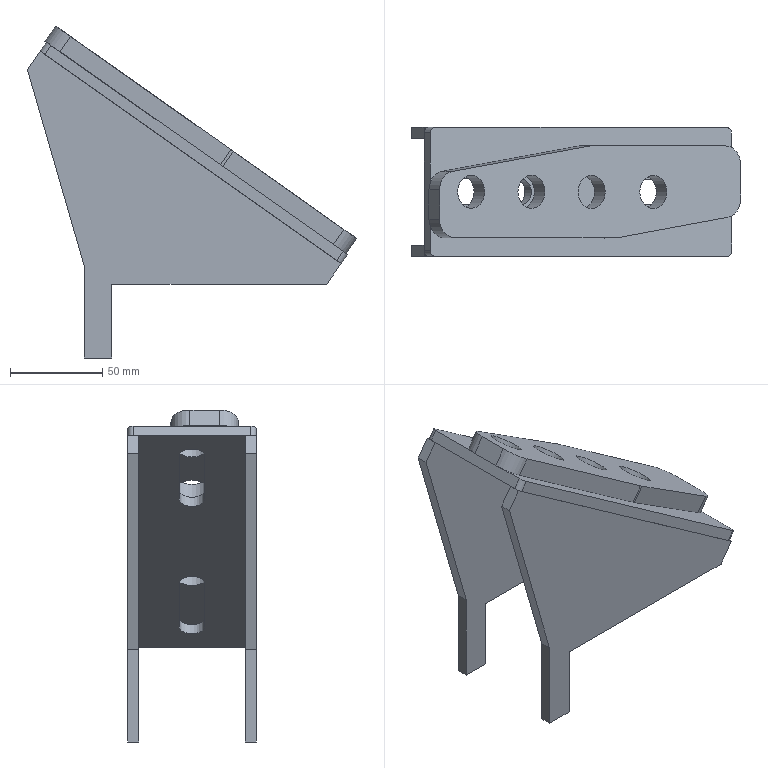Part | STEP file | COMPOUND | 4 solids | 56 faces | box 178.718 x 70 x 180.179 mm | volume 279954 mm3 | plane 38 | cylinder 18 | commonest cylinder face diameters 20 x6 6 x4 14 x4 18 x4